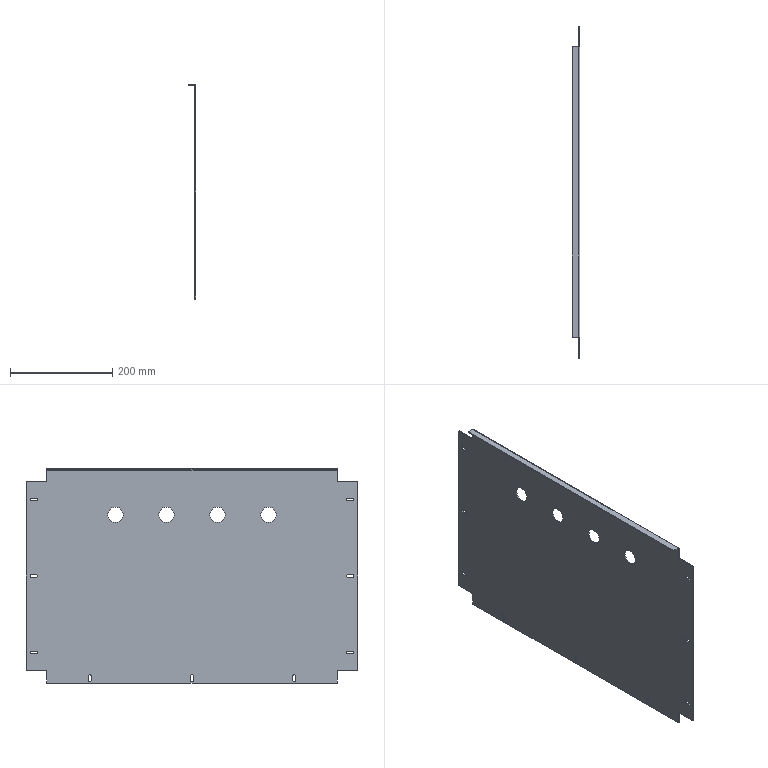Part | SolidWorks | features ICE 4, EdgeFlange 1, FlatPattern 1, HoleWzd 1, SMBaseFlange 1, SheetMetal 1 | 1 solid | 69 faces | box 15 x 650 x 420 mm | volume 545219 mm3 | plane 38 | cylinder 31 | commonest cylinder face diameters 4.5 x21 30 x8 1.473 x1 5.473 x1